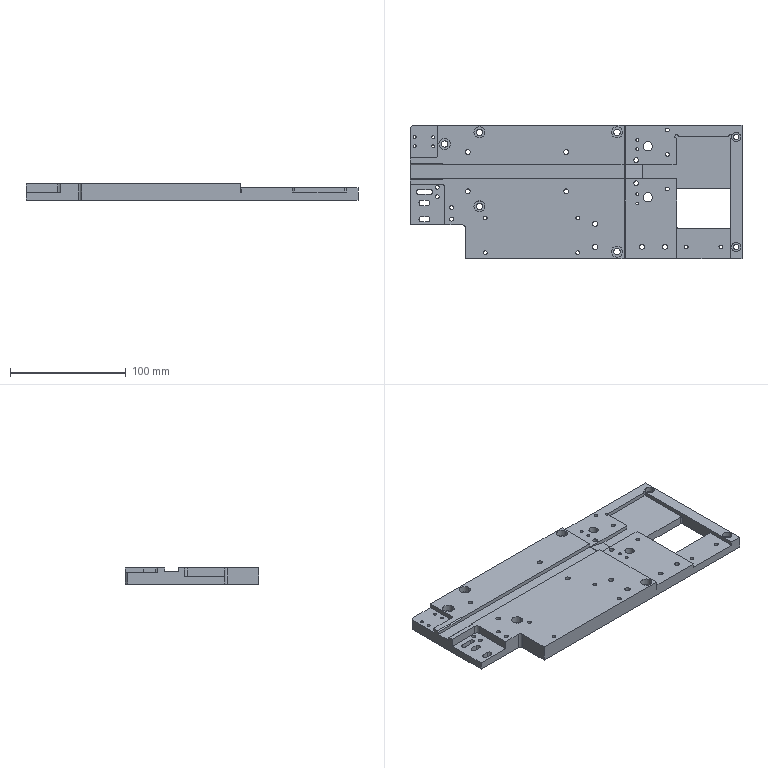Part | STEP file | PN_0004 Mount electronic clip guide groove block | 1 solid | 172 faces | box 287 x 115 x 14 mm | volume 343066 mm3 | cylinder 117 | plane 55 | commonest cylinder face diameters 3.3 x26 2.5 x16 4.2 x16 4.5 x14 8 x12 5.5 x10